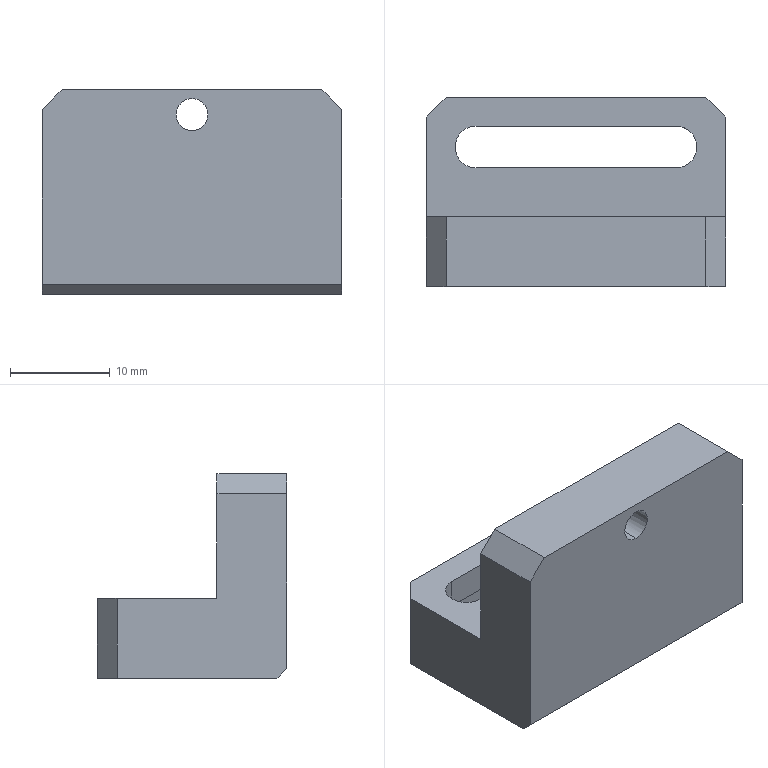Part | SolidWorks | features ICE 4, Chamfer 2, HoleWzd 2, Extrusion 1 | 1 solid | 31 faces | box 30 x 19 x 20.5 mm | volume 5581 mm3 | plane 19 | cylinder 12 | commonest cylinder face diameters 4.2 x3 8 x3 2.5 x2 3.2 x2 3.5 x2
STEP:
#1=CARTESIAN_POINT('',(1.25,-6.,17.001));
#2=VERTEX_POINT('',#1);
#3=CARTESIAN_POINT('',(0.,-7.25,16.4));
#4=VERTEX_POINT('',#3);
#5=CARTESIAN_POINT('',(1.25,-6.,17.001));
#6=CARTESIAN_POINT('',(1.25,-6.086,17.001));
#7=CARTESIAN_POINT('',(1.241,-6.173,16.99));
#8=CARTESIAN_POINT('',(1.206,-6.338,16.949));
#9=CARTESIAN_POINT('',(1.182,-6.415,16.92));
#10=CARTESIAN_POINT('',(1.087,-6.637,16.823));
#11=CARTESIAN_POINT('',(1.001,-6.765,16.745));
#12=CARTESIAN_POINT('',(0.7798,-6.99,16.597));
#13=CARTESIAN_POINT('',(0.6505,-7.08,16.529));
#14=CARTESIAN_POINT('',(0.4204,-7.18,16.454));
#15=CARTESIAN_POINT('',(0.3405,-7.206,16.434));
#16=CARTESIAN_POINT('',(0.1734,-7.241,16.407));
#17=CARTESIAN_POINT('',(0.08602,-7.25,16.4));
#18=CARTESIAN_POINT('',(0.,-7.25,16.4));
#19=B_SPLINE_CURVE_WITH_KNOTS('',3,(#5,#6,#7,#8,#9,#10,#11,#12,#13,#14,#15,#16,#17,#18),.UNSPECIFIED.,.F.,.F.,(4,2,2,2,2,2,4),(0.002061,0.002319,0.002576,0.003092,0.003607,0.003864,0.004122),.UNSPECIFIED.);
#20=EDGE_CURVE('',#2,#4,#19,.T.);
#21=ORIENTED_EDGE('',*,*,#20,.F.);
#22=CARTESIAN_POINT('',(1.25,-6.,10.));
#23=VERTEX_POINT('',#22);
#24=CARTESIAN_POINT('',(1.25,-6.,10.));
#25=DIRECTION('',(0.,0.,-1.));
#26=VECTOR('',#25,1000.);
#27=LINE('',#24,#26);
#28=EDGE_CURVE('',#2,#23,#27,.T.);
#29=ORIENTED_EDGE('',*,*,#28,.T.);
#30=CARTESIAN_POINT('',(-1.25,-6.,10.));
#31=VERTEX_POINT('',#30);
#32=CARTESIAN_POINT('',(0.,-6.,10.));
#33=DIRECTION('',(0.,0.,-1.));
#34=DIRECTION('',(-1.,0.,0.));
#35=AXIS2_PLACEMENT_3D('',#32,#33,#34);
#36=CIRCLE('',#35,1.25);
#37=EDGE_CURVE('',#23,#31,#36,.T.);
#38=ORIENTED_EDGE('',*,*,#37,.T.);
#39=CARTESIAN_POINT('',(-1.25,-6.,17.001));
#40=VERTEX_POINT('',#39);
#41=CARTESIAN_POINT('',(-1.25,-6.,10.));
#42=DIRECTION('',(0.,0.,-1.));
#43=VECTOR('',#42,1000.);
#44=LINE('',#41,#43);
#45=EDGE_CURVE('',#40,#31,#44,.T.);
#46=ORIENTED_EDGE('',*,*,#45,.F.);
#47=CARTESIAN_POINT('',(0.,-7.25,16.4));
#48=CARTESIAN_POINT('',(-0.08574,-7.25,16.4));
#49=CARTESIAN_POINT('',(-0.1725,-7.241,16.407));
#50=CARTESIAN_POINT('',(-0.3395,-7.206,16.434));
#51=CARTESIAN_POINT('',(-0.4194,-7.18,16.454));
#52=CARTESIAN_POINT('',(-0.6488,-7.081,16.529));
#53=CARTESIAN_POINT('',(-0.781,-6.988,16.597));
#54=CARTESIAN_POINT('',(-0.9998,-6.766,16.744));
#55=CARTESIAN_POINT('',(-1.088,-6.636,16.823));
#56=CARTESIAN_POINT('',(-1.213,-6.343,16.952));
#57=CARTESIAN_POINT('',(-1.25,-6.173,17.001));
#58=CARTESIAN_POINT('',(-1.25,-6.,17.001));
#59=B_SPLINE_CURVE_WITH_KNOTS('',3,(#47,#48,#49,#50,#51,#52,#53,#54,#55,#56,#57,#58),.UNSPECIFIED.,.F.,.F.,(4,2,2,2,2,4),(0.004122,0.004379,0.004636,0.005149,0.005663,0.006177),.UNSPECIFIED.);
#60=EDGE_CURVE('',#4,#40,#59,.T.);
#61=ORIENTED_EDGE('',*,*,#60,.F.);
#62=EDGE_LOOP('',(#21,#29,#38,#46,#61));
#63=FACE_OUTER_BOUND('',#62,.T.);
#64=CARTESIAN_POINT('',(0.,-6.,10.));
#65=DIRECTION('',(0.,0.,-1.));
#66=DIRECTION('',(-1.,0.,0.));
#67=AXIS2_PLACEMENT_3D('',#64,#65,#66);
#68=CYLINDRICAL_SURFACE('',#67,1.25);
#69=ADVANCED_FACE('',(#63),#68,.F.);
#70=CARTESIAN_POINT('',(0.,-2.5,19.6));
#71=VERTEX_POINT('',#70);
#72=CARTESIAN_POINT('',(0.,-2.5,16.4));
#73=VERTEX_POINT('',#72);
#74=CARTESIAN_POINT('',(0.,-2.5,18.));
#75=DIRECTION('',(0.,-1.,0.));
#76=DIRECTION('',(0.,0.,-1.));
#77=AXIS2_PLACEMENT_3D('',#74,#75,#76);
#78=CIRCLE('',#77,1.6);
#79=EDGE_CURVE('',#71,#73,#78,.T.);
#80=ORIENTED_EDGE('',*,*,#79,.F.);
#81=CARTESIAN_POINT('',(0.,-9.5,19.6));
#82=VERTEX_POINT('',#81);
#83=CARTESIAN_POINT('',(0.,-9.5,19.6));
#84=DIRECTION('',(0.,-1.,0.));
#85=VECTOR('',#84,1000.);
#86=LINE('',#83,#85);
#87=EDGE_CURVE('',#71,#82,#86,.T.);
#88=ORIENTED_EDGE('',*,*,#87,.T.);
#89=CARTESIAN_POINT('',(0.,-9.5,16.4));
#90=VERTEX_POINT('',#89);
#91=CARTESIAN_POINT('',(0.,-9.5,18.));
#92=DIRECTION('',(0.,-1.,0.));
#93=DIRECTION('',(0.,0.,-1.));
#94=AXIS2_PLACEMENT_3D('',#91,#92,#93);
#95=CIRCLE('',#94,1.6);
#96=EDGE_CURVE('',#82,#90,#95,.T.);
#97=ORIENTED_EDGE('',*,*,#96,.T.);
#98=CARTESIAN_POINT('',(0.,-9.5,16.4));
#99=DIRECTION('',(0.,-1.,0.));
#100=VECTOR('',#99,1000.);
#101=LINE('',#98,#100);
#102=EDGE_CURVE('',#4,#90,#101,.T.);
#103=ORIENTED_EDGE('',*,*,#102,.F.);
#104=ORIENTED_EDGE('',*,*,#60,.T.);
#105=CARTESIAN_POINT('',(0.,-4.75,16.4));
#106=VERTEX_POINT('',#105);
#107=CARTESIAN_POINT('',(-1.25,-6.,17.001));
#108=CARTESIAN_POINT('',(-1.25,-5.913,17.001));
#109=CARTESIAN_POINT('',(-1.241,-5.828,16.99));
#110=CARTESIAN_POINT('',(-1.206,-5.662,16.949));
#111=CARTESIAN_POINT('',(-1.182,-5.585,16.92));
#112=CARTESIAN_POINT('',(-1.088,-5.363,16.823));
#113=CARTESIAN_POINT('',(-1.001,-5.235,16.745));
#114=CARTESIAN_POINT('',(-0.7808,-5.011,16.597));
#115=CARTESIAN_POINT('',(-0.6506,-4.92,16.529));
#116=CARTESIAN_POINT('',(-0.3461,-4.787,16.43));
#117=CARTESIAN_POINT('',(-0.1743,-4.75,16.4));
#118=CARTESIAN_POINT('',(0.,-4.75,16.4));
#119=B_SPLINE_CURVE_WITH_KNOTS('',3,(#107,#108,#109,#110,#111,#112,#113,#114,#115,#116,#117,#118),.UNSPECIFIED.,.F.,.F.,(4,2,2,2,2,4),(0.006177,0.006434,0.006691,0.007205,0.00772,0.008234),.UNSPECIFIED.);
#120=EDGE_CURVE('',#40,#106,#119,.T.);
#121=ORIENTED_EDGE('',*,*,#120,.T.);
#122=CARTESIAN_POINT('',(0.,-9.5,16.4));
#123=DIRECTION('',(0.,-1.,0.));
#124=VECTOR('',#123,1000.);
#125=LINE('',#122,#124);
#126=EDGE_CURVE('',#73,#106,#125,.T.);
#127=ORIENTED_EDGE('',*,*,#126,.F.);
#128=EDGE_LOOP('',(#80,#88,#97,#103,#104,#121,#127));
#129=FACE_OUTER_BOUND('',#128,.T.);
#130=CARTESIAN_POINT('',(0.,-9.5,18.));
#131=DIRECTION('',(0.,-1.,0.));
#132=DIRECTION('',(0.,0.,-1.));
#133=AXIS2_PLACEMENT_3D('',#130,#131,#132);
#134=CYLINDRICAL_SURFACE('',#133,1.6);
#135=ADVANCED_FACE('',(#129),#134,.F.);
#136=CARTESIAN_POINT('',(1.75,-6.,10.));
#137=VERTEX_POINT('',#136);
#138=CARTESIAN_POINT('',(-1.75,-6.,10.));
#139=VERTEX_POINT('',#138);
#140=CARTESIAN_POINT('',(0.,-6.,10.));
#141=DIRECTION('',(0.,0.,-1.));
#142=DIRECTION('',(-1.,0.,0.));
#143=AXIS2_PLACEMENT_3D('',#140,#141,#142);
#144=CIRCLE('',#143,1.75);
#145=EDGE_CURVE('',#137,#139,#144,.T.);
#146=ORIENTED_EDGE('',*,*,#145,.F.);
#147=CARTESIAN_POINT('',(1.75,-6.,0.));
#148=VERTEX_POINT('',#147);
#149=CARTESIAN_POINT('',(1.75,-6.,10.));
#150=DIRECTION('',(0.,0.,-1.));
#151=VECTOR('',#150,1000.);
#152=LINE('',#149,#151);
#153=EDGE_CURVE('',#137,#148,#152,.T.);
#154=ORIENTED_EDGE('',*,*,#153,.T.);
#155=CARTESIAN_POINT('',(-1.75,-6.,0.));
#156=VERTEX_POINT('',#155);
#157=CARTESIAN_POINT('',(0.,-6.,0.));
#158=DIRECTION('',(0.,0.,-1.));
#159=DIRECTION('',(-1.,0.,0.));
#160=AXIS2_PLACEMENT_3D('',#157,#158,#159);
#161=CIRCLE('',#160,1.75);
#162=EDGE_CURVE('',#148,#156,#161,.T.);
#163=ORIENTED_EDGE('',*,*,#162,.T.);
#164=CARTESIAN_POINT('',(-1.75,-6.,10.));
#165=DIRECTION('',(0.,0.,-1.));
#166=VECTOR('',#165,1000.);
#167=LINE('',#164,#166);
#168=EDGE_CURVE('',#139,#156,#167,.T.);
#169=ORIENTED_EDGE('',*,*,#168,.F.);
#170=EDGE_LOOP('',(#146,#154,#163,#169));
#171=FACE_OUTER_BOUND('',#170,.T.);
#172=CARTESIAN_POINT('',(0.,-6.,10.));
#173=DIRECTION('',(0.,0.,-1.));
#174=DIRECTION('',(-1.,0.,0.));
#175=AXIS2_PLACEMENT_3D('',#172,#173,#174);
#176=CYLINDRICAL_SURFACE('',#175,1.75);
#177=ADVANCED_FACE('',(#171),#176,.F.);
#178=CARTESIAN_POINT('',(-14.,4.5,5.));
#179=VERTEX_POINT('',#178);
#180=CARTESIAN_POINT('',(-10.,8.5,5.));
#181=VERTEX_POINT('',#180);
#182=CARTESIAN_POINT('',(-10.,4.5,5.));
#183=DIRECTION('',(0.,0.,-1.));
#184=DIRECTION('',(-1.,0.,0.));
#185=AXIS2_PLACEMENT_3D('',#182,#183,#184);
#186=CIRCLE('',#185,4.);
#187=EDGE_CURVE('',#179,#181,#186,.T.);
#188=ORIENTED_EDGE('',*,*,#187,.F.);
#189=CARTESIAN_POINT('',(-14.,4.5,0.));
#190=VERTEX_POINT('',#189);
#191=CARTESIAN_POINT('',(-14.,4.5,5.));
#192=DIRECTION('',(0.,0.,-1.));
#193=VECTOR('',#192,1000.);
#194=LINE('',#191,#193);
#195=EDGE_CURVE('',#179,#190,#194,.T.);
#196=ORIENTED_EDGE('',*,*,#195,.T.);
#197=CARTESIAN_POINT('',(-10.,8.5,0.));
#198=VERTEX_POINT('',#197);
#199=CARTESIAN_POINT('',(-10.,4.5,0.));
#200=DIRECTION('',(0.,0.,-1.));
#201=DIRECTION('',(-1.,0.,0.));
#202=AXIS2_PLACEMENT_3D('',#199,#200,#201);
#203=CIRCLE('',#202,4.);
#204=EDGE_CURVE('',#190,#198,#203,.T.);
#205=ORIENTED_EDGE('',*,*,#204,.T.);
#206=CARTESIAN_POINT('',(-10.,8.5,5.));
#207=DIRECTION('',(0.,0.,-1.));
#208=VECTOR('',#207,1000.);
#209=LINE('',#206,#208);
#210=EDGE_CURVE('',#181,#198,#209,.T.);
#211=ORIENTED_EDGE('',*,*,#210,.F.);
#212=EDGE_LOOP('',(#188,#196,#205,#211));
#213=FACE_OUTER_BOUND('',#212,.T.);
#214=CARTESIAN_POINT('',(-10.,4.5,5.));
#215=DIRECTION('',(0.,0.,-1.));
#216=DIRECTION('',(-1.,0.,0.));
#217=AXIS2_PLACEMENT_3D('',#214,#215,#216);
#218=CYLINDRICAL_SURFACE('',#217,4.);
#219=ADVANCED_FACE('',(#213),#218,.F.);
#220=CARTESIAN_POINT('',(-10.,6.6,8.));
#221=VERTEX_POINT('',#220);
#222=CARTESIAN_POINT('',(-12.1,4.5,8.));
#223=VERTEX_POINT('',#222);
#224=CARTESIAN_POINT('',(-10.,4.5,8.));
#225=DIRECTION('',(0.,0.,1.));
#226=DIRECTION('',(1.,0.,0.));
#227=AXIS2_PLACEMENT_3D('',#224,#225,#226);
#228=CIRCLE('',#227,2.1);
#229=EDGE_CURVE('',#221,#223,#228,.T.);
#230=ORIENTED_EDGE('',*,*,#229,.T.);
#231=CARTESIAN_POINT('',(-12.1,4.5,5.));
#232=VERTEX_POINT('',#231);
#233=CARTESIAN_POINT('',(-12.1,4.5,20.5));
#234=DIRECTION('',(0.,0.,-1.));
#235=VECTOR('',#234,1000.);
#236=LINE('',#233,#235);
#237=EDGE_CURVE('',#223,#232,#236,.T.);
#238=ORIENTED_EDGE('',*,*,#237,.T.);
#239=CARTESIAN_POINT('',(-10.,6.6,5.));
#240=VERTEX_POINT('',#239);
#241=CARTESIAN_POINT('',(-10.,4.5,5.));
#242=DIRECTION('',(0.,0.,1.));
#243=DIRECTION('',(-1.,0.,0.));
#244=AXIS2_PLACEMENT_3D('',#241,#242,#243);
#245=CIRCLE('',#244,2.1);
#246=EDGE_CURVE('',#240,#232,#245,.T.);
#247=ORIENTED_EDGE('',*,*,#246,.F.);
#248=CARTESIAN_POINT('',(-10.,6.6,20.5));
#249=DIRECTION('',(0.,0.,-1.));
#250=VECTOR('',#249,1000.);
#251=LINE('',#248,#250);
#252=EDGE_CURVE('',#221,#240,#251,.T.);
#253=ORIENTED_EDGE('',*,*,#252,.F.);
#254=EDGE_LOOP('',(#230,#238,#247,#253));
#255=FACE_OUTER_BOUND('',#254,.T.);
#256=CARTESIAN_POINT('',(-10.,4.5,20.5));
#257=DIRECTION('',(0.,0.,-1.));
#258=DIRECTION('',(-1.,0.,0.));
#259=AXIS2_PLACEMENT_3D('',#256,#257,#258);
#260=CYLINDRICAL_SURFACE('',#259,2.1);
#261=ADVANCED_FACE('',(#255),#260,.F.);
#262=ORIENTED_EDGE('',*,*,#237,.F.);
#263=CARTESIAN_POINT('',(-10.,2.4,8.));
#264=VERTEX_POINT('',#263);
#265=CARTESIAN_POINT('',(-10.,4.5,8.));
#266=DIRECTION('',(0.,0.,1.));
#267=DIRECTION('',(1.,0.,0.));
#268=AXIS2_PLACEMENT_3D('',#265,#266,#267);
#269=CIRCLE('',#268,2.1);
#270=EDGE_CURVE('',#223,#264,#269,.T.);
#271=ORIENTED_EDGE('',*,*,#270,.T.);
#272=CARTESIAN_POINT('',(-10.,2.4,5.));
#273=VERTEX_POINT('',#272);
#274=CARTESIAN_POINT('',(-10.,2.4,20.5));
#275=DIRECTION('',(0.,0.,-1.));
#276=VECTOR('',#275,1000.);
#277=LINE('',#274,#276);
#278=EDGE_CURVE('',#264,#273,#277,.T.);
#279=ORIENTED_EDGE('',*,*,#278,.T.);
#280=CARTESIAN_POINT('',(-10.,4.5,5.));
#281=DIRECTION('',(0.,0.,1.));
#282=DIRECTION('',(-1.,0.,0.));
#283=AXIS2_PLACEMENT_3D('',#280,#281,#282);
#284=CIRCLE('',#283,2.1);
#285=EDGE_CURVE('',#232,#273,#284,.T.);
#286=ORIENTED_EDGE('',*,*,#285,.F.);
#287=EDGE_LOOP('',(#262,#271,#279,#286));
#288=FACE_OUTER_BOUND('',#287,.T.);
#289=CARTESIAN_POINT('',(-10.,4.5,20.5));
#290=DIRECTION('',(0.,0.,-1.));
#291=DIRECTION('',(-1.,0.,0.));
#292=AXIS2_PLACEMENT_3D('',#289,#290,#291);
#293=CYLINDRICAL_SURFACE('',#292,2.1);
#294=ADVANCED_FACE('',(#288),#293,.F.);
#295=CARTESIAN_POINT('',(10.,2.4,5.));
#296=VERTEX_POINT('',#295);
#297=CARTESIAN_POINT('',(-10.,2.4,5.));
#298=DIRECTION('',(1.,0.,0.));
#299=VECTOR('',#298,1000.);
#300=LINE('',#297,#299);
#301=EDGE_CURVE('',#273,#296,#300,.T.);
#302=ORIENTED_EDGE('',*,*,#301,.F.);
#303=ORIENTED_EDGE('',*,*,#278,.F.);
#304=CARTESIAN_POINT('',(10.,2.4,8.));
#305=VERTEX_POINT('',#304);
#306=CARTESIAN_POINT('',(0.,2.4,8.));
#307=DIRECTION('',(1.,0.,0.));
#308=VECTOR('',#307,1000.);
#309=LINE('',#306,#308);
#310=EDGE_CURVE('',#264,#305,#309,.T.);
#311=ORIENTED_EDGE('',*,*,#310,.T.);
#312=CARTESIAN_POINT('',(10.,2.4,20.5));
#313=DIRECTION('',(0.,0.,-1.));
#314=VECTOR('',#313,1000.);
#315=LINE('',#312,#314);
#316=EDGE_CURVE('',#305,#296,#315,.T.);
#317=ORIENTED_EDGE('',*,*,#316,.T.);
#318=EDGE_LOOP('',(#302,#303,#311,#317));
#319=FACE_OUTER_BOUND('',#318,.T.);
#320=CARTESIAN_POINT('',(-10.,2.4,20.5));
#321=DIRECTION('',(0.,-1.,0.));
#322=DIRECTION('',(1.,0.,0.));
#323=AXIS2_PLACEMENT_3D('',#320,#321,#322);
#324=PLANE('',#323);
#325=ADVANCED_FACE('',(#319),#324,.F.);
#326=CARTESIAN_POINT('',(10.,6.6,5.));
#327=VERTEX_POINT('',#326);
#328=CARTESIAN_POINT('',(10.,4.5,5.));
#329=DIRECTION('',(0.,0.,1.));
#330=DIRECTION('',(-1.,0.,0.));
#331=AXIS2_PLACEMENT_3D('',#328,#329,#330);
#332=CIRCLE('',#331,2.1);
#333=EDGE_CURVE('',#296,#327,#332,.T.);
#334=ORIENTED_EDGE('',*,*,#333,.F.);
#335=ORIENTED_EDGE('',*,*,#316,.F.);
#336=CARTESIAN_POINT('',(10.,6.6,8.));
#337=VERTEX_POINT('',#336);
#338=CARTESIAN_POINT('',(10.,4.5,8.));
#339=DIRECTION('',(0.,0.,1.));
#340=DIRECTION('',(1.,0.,0.));
#341=AXIS2_PLACEMENT_3D('',#338,#339,#340);
#342=CIRCLE('',#341,2.1);
#343=EDGE_CURVE('',#305,#337,#342,.T.);
#344=ORIENTED_EDGE('',*,*,#343,.T.);
#345=CARTESIAN_POINT('',(10.,6.6,20.5));
#346=DIRECTION('',(0.,0.,-1.));
#347=VECTOR('',#346,1000.);
#348=LINE('',#345,#347);
#349=EDGE_CURVE('',#337,#327,#348,.T.);
#350=ORIENTED_EDGE('',*,*,#349,.T.);
#351=EDGE_LOOP('',(#334,#335,#344,#350));
#352=FACE_OUTER_BOUND('',#351,.T.);
#353=CARTESIAN_POINT('',(10.,4.5,20.5));
#354=DIRECTION('',(0.,0.,-1.));
#355=DIRECTION('',(-1.,0.,0.));
#356=AXIS2_PLACEMENT_3D('',#353,#354,#355);
#357=CYLINDRICAL_SURFACE('',#356,2.1);
#358=ADVANCED_FACE('',(#352),#357,.F.);
#359=CARTESIAN_POINT('',(-10.,6.6,5.));
#360=DIRECTION('',(-1.,0.,0.));
#361=VECTOR('',#360,1000.);
#362=LINE('',#359,#361);
#363=EDGE_CURVE('',#327,#240,#362,.T.);
#364=ORIENTED_EDGE('',*,*,#363,.F.);
#365=ORIENTED_EDGE('',*,*,#349,.F.);
#366=CARTESIAN_POINT('',(0.,6.6,8.));
#367=DIRECTION('',(-1.,0.,0.));
#368=VECTOR('',#367,1000.);
#369=LINE('',#366,#368);
#370=EDGE_CURVE('',#337,#221,#369,.T.);
#371=ORIENTED_EDGE('',*,*,#370,.T.);
#372=ORIENTED_EDGE('',*,*,#252,.T.);
#373=EDGE_LOOP('',(#364,#365,#371,#372));
#374=FACE_OUTER_BOUND('',#373,.T.);
#375=CARTESIAN_POINT('',(-10.,6.6,20.5));
#376=DIRECTION('',(0.,1.,0.));
#377=DIRECTION('',(-1.,0.,0.));
#378=AXIS2_PLACEMENT_3D('',#375,#376,#377);
#379=PLANE('',#378);
#380=ADVANCED_FACE('',(#374),#379,.F.);
#381=CARTESIAN_POINT('',(13.,9.5,0.));
#382=VERTEX_POINT('',#381);
#383=CARTESIAN_POINT('',(-13.,9.5,0.));
#384=VERTEX_POINT('',#383);
#385=CARTESIAN_POINT('',(-15.,9.5,0.));
#386=DIRECTION('',(-1.,0.,0.));
#387=VECTOR('',#386,1000.);
#388=LINE('',#385,#387);
#389=EDGE_CURVE('',#382,#384,#388,.T.);
#390=ORIENTED_EDGE('',*,*,#389,.T.);
#391=CARTESIAN_POINT('',(-13.,9.5,8.));
#392=VERTEX_POINT('',#391);
#393=CARTESIAN_POINT('',(-13.,9.5,20.5));
#394=DIRECTION('',(0.,0.,1.));
#395=VECTOR('',#394,1000.);
#396=LINE('',#393,#395);
#397=EDGE_CURVE('',#384,#392,#396,.T.);
#398=ORIENTED_EDGE('',*,*,#397,.T.);
#399=CARTESIAN_POINT('',(13.,9.5,8.));
#400=VERTEX_POINT('',#399);
#401=CARTESIAN_POINT('',(-15.,9.5,8.));
#402=DIRECTION('',(-1.,0.,0.));
#403=VECTOR('',#402,1000.);
#404=LINE('',#401,#403);
#405=EDGE_CURVE('',#400,#392,#404,.T.);
#406=ORIENTED_EDGE('',*,*,#405,.F.);
#407=CARTESIAN_POINT('',(13.,9.5,20.5));
#408=DIRECTION('',(0.,0.,-1.));
#409=VECTOR('',#408,1000.);
#410=LINE('',#407,#409);
#411=EDGE_CURVE('',#400,#382,#410,.T.);
#412=ORIENTED_EDGE('',*,*,#411,.T.);
#413=EDGE_LOOP('',(#390,#398,#406,#412));
#414=FACE_OUTER_BOUND('',#413,.T.);
#415=CARTESIAN_POINT('',(-15.,9.5,20.5));
#416=DIRECTION('',(0.,-1.,0.));
#417=DIRECTION('',(0.,0.,-1.));
#418=AXIS2_PLACEMENT_3D('',#415,#416,#417);
#419=PLANE('',#418);
#420=ADVANCED_FACE('',(#414),#419,.F.);
#421=CARTESIAN_POINT('',(15.,-9.5,18.5));
#422=VERTEX_POINT('',#421);
#423=CARTESIAN_POINT('',(15.,-9.5,1.));
#424=VERTEX_POINT('',#423);
#425=CARTESIAN_POINT('',(15.,-9.5,20.5));
#426=DIRECTION('',(0.,0.,-1.));
#427=VECTOR('',#426,1000.);
#428=LINE('',#425,#427);
#429=EDGE_CURVE('',#422,#424,#428,.T.);
#430=ORIENTED_EDGE('',*,*,#429,.T.);
#431=CARTESIAN_POINT('',(15.,-8.5,0.));
#432=VERTEX_POINT('',#431);
#433=CARTESIAN_POINT('',(15.,-9.5,1.));
#434=DIRECTION('',(0.,0.7071,-0.7071));
#435=VECTOR('',#434,1000.);
#436=LINE('',#433,#435);
#437=EDGE_CURVE('',#424,#432,#436,.T.);
#438=ORIENTED_EDGE('',*,*,#437,.T.);
#439=CARTESIAN_POINT('',(15.,7.5,0.));
#440=VERTEX_POINT('',#439);
#441=CARTESIAN_POINT('',(15.,-9.5,0.));
#442=DIRECTION('',(0.,1.,0.));
#443=VECTOR('',#442,1000.);
#444=LINE('',#441,#443);
#445=EDGE_CURVE('',#432,#440,#444,.T.);
#446=ORIENTED_EDGE('',*,*,#445,.T.);
#447=CARTESIAN_POINT('',(15.,7.5,8.));
#448=VERTEX_POINT('',#447);
#449=CARTESIAN_POINT('',(15.,7.5,20.5));
#450=DIRECTION('',(0.,0.,1.));
#451=VECTOR('',#450,1000.);
#452=LINE('',#449,#451);
#453=EDGE_CURVE('',#440,#448,#452,.T.);
#454=ORIENTED_EDGE('',*,*,#453,.T.);
#455=CARTESIAN_POINT('',(15.,-2.5,8.));
#456=VERTEX_POINT('',#455);
#457=CARTESIAN_POINT('',(15.,9.5,8.));
#458=DIRECTION('',(0.,1.,0.));
#459=VECTOR('',#458,1000.);
#460=LINE('',#457,#459);
#461=EDGE_CURVE('',#456,#448,#460,.T.);
#462=ORIENTED_EDGE('',*,*,#461,.F.);
#463=CARTESIAN_POINT('',(15.,-2.5,18.5));
#464=VERTEX_POINT('',#463);
#465=CARTESIAN_POINT('',(15.,-2.5,8.));
#466=DIRECTION('',(0.,0.,1.));
#467=VECTOR('',#466,1000.);
#468=LINE('',#465,#467);
#469=EDGE_CURVE('',#456,#464,#468,.T.);
#470=ORIENTED_EDGE('',*,*,#469,.T.);
#471=CARTESIAN_POINT('',(15.,-9.5,18.5));
#472=DIRECTION('',(0.,-1.,0.));
#473=VECTOR('',#472,1000.);
#474=LINE('',#471,#473);
#475=EDGE_CURVE('',#464,#422,#474,.T.);
#476=ORIENTED_EDGE('',*,*,#475,.T.);
#477=EDGE_LOOP('',(#430,#438,#446,#454,#462,#470,#476));
#478=FACE_OUTER_BOUND('',#477,.T.);
#479=CARTESIAN_POINT('',(15.,-9.5,20.5));
#480=DIRECTION('',(-1.,0.,0.));
#481=DIRECTION('',(0.,0.,1.));
#482=AXIS2_PLACEMENT_3D('',#479,#480,#481);
#483=PLANE('',#482);
#484=ADVANCED_FACE('',(#478),#483,.F.);
#485=CARTESIAN_POINT('',(-15.,7.5,0.));
#486=VERTEX_POINT('',#485);
#487=CARTESIAN_POINT('',(-15.,-8.5,0.));
#488=VERTEX_POINT('',#487);
#489=CARTESIAN_POINT('',(-15.,-9.5,0.));
#490=DIRECTION('',(0.,-1.,0.));
#491=VECTOR('',#490,1000.);
#492=LINE('',#489,#491);
#493=EDGE_CURVE('',#486,#488,#492,.T.);
#494=ORIENTED_EDGE('',*,*,#493,.T.);
#495=CARTESIAN_POINT('',(-15.,-9.5,1.));
#496=VERTEX_POINT('',#495);
#497=CARTESIAN_POINT('',(-15.,-9.5,1.));
#498=DIRECTION('',(0.,-0.7071,0.7071));
#499=VECTOR('',#498,1000.);
#500=LINE('',#497,#499);
#501=EDGE_CURVE('',#488,#496,#500,.T.);
#502=ORIENTED_EDGE('',*,*,#501,.T.);
#503=CARTESIAN_POINT('',(-15.,-9.5,18.5));
#504=VERTEX_POINT('',#503);
#505=CARTESIAN_POINT('',(-15.,-9.5,20.5));
#506=DIRECTION('',(0.,0.,-1.));
#507=VECTOR('',#506,1000.);
#508=LINE('',#505,#507);
#509=EDGE_CURVE('',#504,#496,#508,.T.);
#510=ORIENTED_EDGE('',*,*,#509,.F.);
#511=CARTESIAN_POINT('',(-15.,-2.5,18.5));
#512=VERTEX_POINT('',#511);
#513=CARTESIAN_POINT('',(-15.,-9.5,18.5));
#514=DIRECTION('',(0.,1.,0.));
#515=VECTOR('',#514,1000.);
#516=LINE('',#513,#515);
#517=EDGE_CURVE('',#504,#512,#516,.T.);
#518=ORIENTED_EDGE('',*,*,#517,.T.);
#519=CARTESIAN_POINT('',(-15.,-2.5,8.));
#520=VERTEX_POINT('',#519);
#521=CARTESIAN_POINT('',(-15.,-2.5,8.));
#522=DIRECTION('',(0.,0.,1.));
#523=VECTOR('',#522,1000.);
#524=LINE('',#521,#523);
#525=EDGE_CURVE('',#520,#512,#524,.T.);
#526=ORIENTED_EDGE('',*,*,#525,.F.);
#527=CARTESIAN_POINT('',(-15.,7.5,8.));
#528=VERTEX_POINT('',#527);
#529=CARTESIAN_POINT('',(-15.,9.5,8.));
#530=DIRECTION('',(0.,-1.,0.));
#531=VECTOR('',#530,1000.);
#532=LINE('',#529,#531);
#533=EDGE_CURVE('',#528,#520,#532,.T.);
#534=ORIENTED_EDGE('',*,*,#533,.F.);
#535=CARTESIAN_POINT('',(-15.,7.5,20.5));
#536=DIRECTION('',(0.,0.,-1.));
#537=VECTOR('',#536,1000.);
#538=LINE('',#535,#537);
#539=EDGE_CURVE('',#528,#486,#538,.T.);
#540=ORIENTED_EDGE('',*,*,#539,.T.);
#541=EDGE_LOOP('',(#494,#502,#510,#518,#526,#534,#540));
#542=FACE_OUTER_BOUND('',#541,.T.);
#543=CARTESIAN_POINT('',(-15.,-9.5,20.5));
#544=DIRECTION('',(1.,0.,0.));
#545=DIRECTION('',(0.,0.,-1.));
#546=AXIS2_PLACEMENT_3D('',#543,#544,#545);
#547=PLANE('',#546);
#548=ADVANCED_FACE('',(#542),#547,.F.);
#549=CARTESIAN_POINT('',(0.,-9.5,18.));
#550=DIRECTION('',(0.,-1.,0.));
#551=DIRECTION('',(0.,0.,-1.));
#552=AXIS2_PLACEMENT_3D('',#549,#550,#551);
#553=CIRCLE('',#552,1.6);
#554=EDGE_CURVE('',#90,#82,#553,.T.);
#555=ORIENTED_EDGE('',*,*,#554,.F.);
#556=ORIENTED_EDGE('',*,*,#96,.F.);
#557=EDGE_LOOP('',(#555,#556));
#558=FACE_BOUND('',#557,.T.);
#559=ORIENTED_EDGE('',*,*,#509,.T.);
#560=CARTESIAN_POINT('',(15.,-9.5,1.));
#561=DIRECTION('',(1.,0.,0.));
#562=VECTOR('',#561,1000.);
#563=LINE('',#560,#562);
#564=EDGE_CURVE('',#496,#424,#563,.T.);
#565=ORIENTED_EDGE('',*,*,#564,.T.);
#566=ORIENTED_EDGE('',*,*,#429,.F.);
#567=CARTESIAN_POINT('',(13.,-9.5,20.5));
#568=VERTEX_POINT('',#567);
#569=CARTESIAN_POINT('',(13.,-9.5,20.5));
#570=DIRECTION('',(-0.7071,0.,0.7071));
#571=VECTOR('',#570,1000.);
#572=LINE('',#569,#571);
#573=EDGE_CURVE('',#422,#568,#572,.T.);
#574=ORIENTED_EDGE('',*,*,#573,.T.);
#575=CARTESIAN_POINT('',(-13.,-9.5,20.5));
#576=VERTEX_POINT('',#575);
#577=CARTESIAN_POINT('',(-15.,-9.5,20.5));
#578=DIRECTION('',(1.,0.,0.));
#579=VECTOR('',#578,1000.);
#580=LINE('',#577,#579);
#581=EDGE_CURVE('',#576,#568,#580,.T.);
#582=ORIENTED_EDGE('',*,*,#581,.F.);
#583=CARTESIAN_POINT('',(-13.,-9.5,20.5));
#584=DIRECTION('',(-0.7071,0.,-0.7071));
#585=VECTOR('',#584,1000.);
#586=LINE('',#583,#585);
#587=EDGE_CURVE('',#576,#504,#586,.T.);
#588=ORIENTED_EDGE('',*,*,#587,.T.);
#589=EDGE_LOOP('',(#559,#565,#566,#574,#582,#588));
#590=FACE_OUTER_BOUND('',#589,.T.);
#591=CARTESIAN_POINT('',(-15.,-9.5,20.5));
#592=DIRECTION('',(0.,1.,0.));
#593=DIRECTION('',(0.,0.,1.));
#594=AXIS2_PLACEMENT_3D('',#591,#592,#593);
#595=PLANE('',#594);
#596=ADVANCED_FACE('',(#558,#590),#595,.F.);
#597=ORIENTED_EDGE('',*,*,#581,.T.);
#598=CARTESIAN_POINT('',(13.,-2.5,20.5));
#599=VERTEX_POINT('',#598);
#600=CARTESIAN_POINT('',(13.,0.,20.5));
#601=DIRECTION('',(0.,1.,0.));
#602=VECTOR('',#601,1000.);
#603=LINE('',#600,#602);
#604=EDGE_CURVE('',#568,#599,#603,.T.);
#605=ORIENTED_EDGE('',*,*,#604,.T.);
#606=CARTESIAN_POINT('',(-13.,-2.5,20.5));
#607=VERTEX_POINT('',#606);
#608=CARTESIAN_POINT('',(-15.,-2.5,20.5));
#609=DIRECTION('',(1.,0.,0.));
#610=VECTOR('',#609,1000.);
#611=LINE('',#608,#610);
#612=EDGE_CURVE('',#607,#599,#611,.T.);
#613=ORIENTED_EDGE('',*,*,#612,.F.);
#614=CARTESIAN_POINT('',(-13.,0.,20.5));
#615=DIRECTION('',(0.,-1.,0.));
#616=VECTOR('',#615,1000.);
#617=LINE('',#614,#616);
#618=EDGE_CURVE('',#607,#576,#617,.T.);
#619=ORIENTED_EDGE('',*,*,#618,.T.);
#620=EDGE_LOOP('',(#597,#605,#613,#619));
#621=FACE_OUTER_BOUND('',#620,.T.);
#622=CARTESIAN_POINT('',(0.,0.,20.5));
#623=DIRECTION('',(0.,0.,-1.));
#624=DIRECTION('',(-1.,0.,0.));
#625=AXIS2_PLACEMENT_3D('',#622,#623,#624);
#626=PLANE('',#625);
#627=ADVANCED_FACE('',(#621),#626,.F.);
#628=CARTESIAN_POINT('',(0.,-6.,0.));
#629=DIRECTION('',(0.,0.,-1.));
#630=DIRECTION('',(-1.,0.,0.));
#631=AXIS2_PLACEMENT_3D('',#628,#629,#630);
#632=CIRCLE('',#631,1.75);
#633=EDGE_CURVE('',#156,#148,#632,.T.);
#634=ORIENTED_EDGE('',*,*,#633,.F.);
#635=ORIENTED_EDGE('',*,*,#162,.F.);
#636=EDGE_LOOP('',(#634,#635));
#637=FACE_BOUND('',#636,.T.);
#638=CARTESIAN_POINT('',(-10.,0.5,0.));
#639=VERTEX_POINT('',#638);
#640=CARTESIAN_POINT('',(-10.,4.5,0.));
#641=DIRECTION('',(0.,0.,-1.));
#642=DIRECTION('',(-1.,0.,0.));
#643=AXIS2_PLACEMENT_3D('',#640,#641,#642);
#644=CIRCLE('',#643,4.);
#645=EDGE_CURVE('',#639,#190,#644,.T.);
#646=ORIENTED_EDGE('',*,*,#645,.F.);
#647=CARTESIAN_POINT('',(10.,0.5,0.));
#648=VERTEX_POINT('',#647);
#649=CARTESIAN_POINT('',(-10.,0.5,0.));
#650=DIRECTION('',(-1.,0.,0.));
#651=VECTOR('',#650,1000.);
#652=LINE('',#649,#651);
#653=EDGE_CURVE('',#648,#639,#652,.T.);
#654=ORIENTED_EDGE('',*,*,#653,.F.);
#655=CARTESIAN_POINT('',(10.,8.5,0.));
#656=VERTEX_POINT('',#655);
#657=CARTESIAN_POINT('',(10.,4.5,0.));
#658=DIRECTION('',(0.,0.,-1.));
#659=DIRECTION('',(-1.,0.,0.));
#660=AXIS2_PLACEMENT_3D('',#657,#658,#659);
#661=CIRCLE('',#660,4.);
#662=EDGE_CURVE('',#656,#648,#661,.T.);
#663=ORIENTED_EDGE('',*,*,#662,.F.);
#664=CARTESIAN_POINT('',(-10.,8.5,0.));
#665=DIRECTION('',(1.,0.,0.));
#666=VECTOR('',#665,1000.);
#667=LINE('',#664,#666);
#668=EDGE_CURVE('',#198,#656,#667,.T.);
#669=ORIENTED_EDGE('',*,*,#668,.F.);
#670=ORIENTED_EDGE('',*,*,#204,.F.);
#671=EDGE_LOOP('',(#646,#654,#663,#669,#670));
#672=FACE_BOUND('',#671,.T.);
#673=ORIENTED_EDGE('',*,*,#445,.F.);
#674=CARTESIAN_POINT('',(-15.,-8.5,0.));
#675=DIRECTION('',(-1.,0.,0.));
#676=VECTOR('',#675,1000.);
#677=LINE('',#674,#676);
#678=EDGE_CURVE('',#432,#488,#677,.T.);
#679=ORIENTED_EDGE('',*,*,#678,.T.);
#680=ORIENTED_EDGE('',*,*,#493,.F.);
#681=CARTESIAN_POINT('',(-11.25,11.25,0.));
#682=DIRECTION('',(0.7071,0.7071,0.));
#683=VECTOR('',#682,1000.);
#684=LINE('',#681,#683);
#685=EDGE_CURVE('',#486,#384,#684,.T.);
#686=ORIENTED_EDGE('',*,*,#685,.T.);
#687=ORIENTED_EDGE('',*,*,#389,.F.);
#688=CARTESIAN_POINT('',(11.25,11.25,0.));
#689=DIRECTION('',(0.7071,-0.7071,0.));
#690=VECTOR('',#689,1000.);
#691=LINE('',#688,#690);
#692=EDGE_CURVE('',#382,#440,#691,.T.);
#693=ORIENTED_EDGE('',*,*,#692,.T.);
#694=EDGE_LOOP('',(#673,#679,#680,#686,#687,#693));
#695=FACE_OUTER_BOUND('',#694,.T.);
#696=CARTESIAN_POINT('',(0.,0.,0.));
#697=DIRECTION('',(0.,0.,-1.));
#698=DIRECTION('',(-1.,0.,0.));
#699=AXIS2_PLACEMENT_3D('',#696,#697,#698);
#700=PLANE('',#699);
#701=ADVANCED_FACE('',(#637,#672,#695),#700,.T.);
#702=CARTESIAN_POINT('',(0.,-2.5,18.));
#703=DIRECTION('',(0.,-1.,0.));
#704=DIRECTION('',(0.,0.,-1.));
#705=AXIS2_PLACEMENT_3D('',#702,#703,#704);
#706=CIRCLE('',#705,1.6);
#707=EDGE_CURVE('',#73,#71,#706,.T.);
#708=ORIENTED_EDGE('',*,*,#707,.T.);
#709=ORIENTED_EDGE('',*,*,#79,.T.);
#710=EDGE_LOOP('',(#708,#709));
#711=FACE_BOUND('',#710,.T.);
#712=ORIENTED_EDGE('',*,*,#612,.T.);
#713=CARTESIAN_POINT('',(13.,-2.5,20.5));
#714=DIRECTION('',(0.7071,0.,-0.7071));
#715=VECTOR('',#714,1000.);
#716=LINE('',#713,#715);
#717=EDGE_CURVE('',#599,#464,#716,.T.);
#718=ORIENTED_EDGE('',*,*,#717,.T.);
#719=ORIENTED_EDGE('',*,*,#469,.F.);
#720=CARTESIAN_POINT('',(-15.,-2.5,8.));
#721=DIRECTION('',(1.,0.,0.));
#722=VECTOR('',#721,1000.);
#723=LINE('',#720,#722);
#724=EDGE_CURVE('',#520,#456,#723,.T.);
#725=ORIENTED_EDGE('',*,*,#724,.F.);
#726=ORIENTED_EDGE('',*,*,#525,.T.);
#727=CARTESIAN_POINT('',(-13.,-2.5,20.5));
#728=DIRECTION('',(0.7071,0.,0.7071));
#729=VECTOR('',#728,1000.);
#730=LINE('',#727,#729);
#731=EDGE_CURVE('',#512,#607,#730,.T.);
#732=ORIENTED_EDGE('',*,*,#731,.T.);
#733=EDGE_LOOP('',(#712,#718,#719,#725,#726,#732));
#734=FACE_OUTER_BOUND('',#733,.T.);
#735=CARTESIAN_POINT('',(-15.,-2.5,8.));
#736=DIRECTION('',(0.,-1.,0.));
#737=DIRECTION('',(0.,0.,-1.));
#738=AXIS2_PLACEMENT_3D('',#735,#736,#737);
#739=PLANE('',#738);
#740=ADVANCED_FACE('',(#711,#734),#739,.F.);
#741=ORIENTED_EDGE('',*,*,#229,.F.);
#742=ORIENTED_EDGE('',*,*,#370,.F.);
#743=ORIENTED_EDGE('',*,*,#343,.F.);
#744=ORIENTED_EDGE('',*,*,#310,.F.);
#745=ORIENTED_EDGE('',*,*,#270,.F.);
#746=EDGE_LOOP('',(#741,#742,#743,#744,#745));
#747=FACE_BOUND('',#746,.T.);
#748=ORIENTED_EDGE('',*,*,#405,.T.);
#749=CARTESIAN_POINT('',(-11.25,11.25,8.));
#750=DIRECTION('',(-0.7071,-0.7071,0.));
#751=VECTOR('',#750,1000.);
#752=LINE('',#749,#751);
#753=EDGE_CURVE('',#392,#528,#752,.T.);
#754=ORIENTED_EDGE('',*,*,#753,.T.);
#755=ORIENTED_EDGE('',*,*,#533,.T.);
#756=ORIENTED_EDGE('',*,*,#724,.T.);
#757=ORIENTED_EDGE('',*,*,#461,.T.);
#758=CARTESIAN_POINT('',(11.25,11.25,8.));
#759=DIRECTION('',(-0.7071,0.7071,0.));
#760=VECTOR('',#759,1000.);
#761=LINE('',#758,#760);
#762=EDGE_CURVE('',#448,#400,#761,.T.);
#763=ORIENTED_EDGE('',*,*,#762,.T.);
#764=EDGE_LOOP('',(#748,#754,#755,#756,#757,#763));
#765=FACE_OUTER_BOUND('',#764,.T.);
#766=CARTESIAN_POINT('',(0.,0.,8.));
#767=DIRECTION('',(0.,0.,1.));
#768=DIRECTION('',(1.,0.,0.));
#769=AXIS2_PLACEMENT_3D('',#766,#767,#768);
#770=PLANE('',#769);
#771=ADVANCED_FACE('',(#747,#765),#770,.T.);
#772=CARTESIAN_POINT('',(-10.,0.5,5.));
#773=VERTEX_POINT('',#772);
#774=CARTESIAN_POINT('',(-10.,4.5,5.));
#775=DIRECTION('',(0.,0.,-1.));
#776=DIRECTION('',(-1.,0.,0.));
#777=AXIS2_PLACEMENT_3D('',#774,#775,#776);
#778=CIRCLE('',#777,4.);
#779=EDGE_CURVE('',#773,#179,#778,.T.);
#780=ORIENTED_EDGE('',*,*,#779,.T.);
#781=ORIENTED_EDGE('',*,*,#187,.T.);
#782=CARTESIAN_POINT('',(10.,8.5,5.));
#783=VERTEX_POINT('',#782);
#784=CARTESIAN_POINT('',(-10.,8.5,5.));
#785=DIRECTION('',(1.,0.,0.));
#786=VECTOR('',#785,1000.);
#787=LINE('',#784,#786);
#788=EDGE_CURVE('',#181,#783,#787,.T.);
#789=ORIENTED_EDGE('',*,*,#788,.T.);
#790=CARTESIAN_POINT('',(10.,0.5,5.));
#791=VERTEX_POINT('',#790);
#792=CARTESIAN_POINT('',(10.,4.5,5.));
#793=DIRECTION('',(0.,0.,-1.));
#794=DIRECTION('',(-1.,0.,0.));
#795=AXIS2_PLACEMENT_3D('',#792,#793,#794);
#796=CIRCLE('',#795,4.);
#797=EDGE_CURVE('',#783,#791,#796,.T.);
#798=ORIENTED_EDGE('',*,*,#797,.T.);
#799=CARTESIAN_POINT('',(-10.,0.5,5.));
#800=DIRECTION('',(-1.,0.,0.));
#801=VECTOR('',#800,1000.);
#802=LINE('',#799,#801);
#803=EDGE_CURVE('',#791,#773,#802,.T.);
#804=ORIENTED_EDGE('',*,*,#803,.T.);
#805=EDGE_LOOP('',(#780,#781,#789,#798,#804));
#806=FACE_OUTER_BOUND('',#805,.T.);
#807=ORIENTED_EDGE('',*,*,#246,.T.);
#808=ORIENTED_EDGE('',*,*,#285,.T.);
#809=ORIENTED_EDGE('',*,*,#301,.T.);
#810=ORIENTED_EDGE('',*,*,#333,.T.);
#811=ORIENTED_EDGE('',*,*,#363,.T.);
#812=EDGE_LOOP('',(#807,#808,#809,#810,#811));
#813=FACE_BOUND('',#812,.T.);
#814=CARTESIAN_POINT('',(-10.,4.5,5.));
#815=DIRECTION('',(0.,0.,-1.));
#816=DIRECTION('',(-1.,0.,0.));
#817=AXIS2_PLACEMENT_3D('',#814,#815,#816);
#818=PLANE('',#817);
#819=ADVANCED_FACE('',(#806,#813),#818,.T.);
#820=ORIENTED_EDGE('',*,*,#195,.F.);
#821=ORIENTED_EDGE('',*,*,#779,.F.);
#822=CARTESIAN_POINT('',(-10.,0.5,5.));
#823=DIRECTION('',(0.,0.,-1.));
#824=VECTOR('',#823,1000.);
#825=LINE('',#822,#824);
#826=EDGE_CURVE('',#773,#639,#825,.T.);
#827=ORIENTED_EDGE('',*,*,#826,.T.);
#828=ORIENTED_EDGE('',*,*,#645,.T.);
#829=EDGE_LOOP('',(#820,#821,#827,#828));
#830=FACE_OUTER_BOUND('',#829,.T.);
#831=CARTESIAN_POINT('',(-10.,4.5,5.));
#832=DIRECTION('',(0.,0.,-1.));
#833=DIRECTION('',(-1.,0.,0.));
#834=AXIS2_PLACEMENT_3D('',#831,#832,#833);
#835=CYLINDRICAL_SURFACE('',#834,4.);
#836=ADVANCED_FACE('',(#830),#835,.F.);
#837=ORIENTED_EDGE('',*,*,#653,.T.);
#838=ORIENTED_EDGE('',*,*,#826,.F.);
#839=ORIENTED_EDGE('',*,*,#803,.F.);
#840=CARTESIAN_POINT('',(10.,0.5,5.));
#841=DIRECTION('',(0.,0.,-1.));
#842=VECTOR('',#841,1000.);
#843=LINE('',#840,#842);
#844=EDGE_CURVE('',#791,#648,#843,.T.);
#845=ORIENTED_EDGE('',*,*,#844,.T.);
#846=EDGE_LOOP('',(#837,#838,#839,#845));
#847=FACE_OUTER_BOUND('',#846,.T.);
#848=CARTESIAN_POINT('',(-10.,0.5,5.));
#849=DIRECTION('',(0.,-1.,0.));
#850=DIRECTION('',(1.,0.,0.));
#851=AXIS2_PLACEMENT_3D('',#848,#849,#850);
#852=PLANE('',#851);
#853=ADVANCED_FACE('',(#847),#852,.F.);
#854=ORIENTED_EDGE('',*,*,#662,.T.);
#855=ORIENTED_EDGE('',*,*,#844,.F.);
#856=ORIENTED_EDGE('',*,*,#797,.F.);
#857=CARTESIAN_POINT('',(10.,8.5,5.));
#858=DIRECTION('',(0.,0.,-1.));
#859=VECTOR('',#858,1000.);
#860=LINE('',#857,#859);
#861=EDGE_CURVE('',#783,#656,#860,.T.);
#862=ORIENTED_EDGE('',*,*,#861,.T.);
#863=EDGE_LOOP('',(#854,#855,#856,#862));
#864=FACE_OUTER_BOUND('',#863,.T.);
#865=CARTESIAN_POINT('',(10.,4.5,5.));
#866=DIRECTION('',(0.,0.,-1.));
#867=DIRECTION('',(-1.,0.,0.));
#868=AXIS2_PLACEMENT_3D('',#865,#866,#867);
#869=CYLINDRICAL_SURFACE('',#868,4.);
#870=ADVANCED_FACE('',(#864),#869,.F.);
#871=ORIENTED_EDGE('',*,*,#668,.T.);
#872=ORIENTED_EDGE('',*,*,#861,.F.);
#873=ORIENTED_EDGE('',*,*,#788,.F.);
#874=ORIENTED_EDGE('',*,*,#210,.T.);
#875=EDGE_LOOP('',(#871,#872,#873,#874));
#876=FACE_OUTER_BOUND('',#875,.T.);
#877=CARTESIAN_POINT('',(-10.,8.5,5.));
#878=DIRECTION('',(0.,1.,0.));
#879=DIRECTION('',(-1.,0.,0.));
#880=AXIS2_PLACEMENT_3D('',#877,#878,#879);
#881=PLANE('',#880);
#882=ADVANCED_FACE('',(#876),#881,.F.);
#883=ORIENTED_EDGE('',*,*,#153,.F.);
#884=CARTESIAN_POINT('',(0.,-6.,10.));
#885=DIRECTION('',(0.,0.,-1.));
#886=DIRECTION('',(-1.,0.,0.));
#887=AXIS2_PLACEMENT_3D('',#884,#885,#886);
#888=CIRCLE('',#887,1.75);
#889=EDGE_CURVE('',#139,#137,#888,.T.);
#890=ORIENTED_EDGE('',*,*,#889,.F.);
#891=ORIENTED_EDGE('',*,*,#168,.T.);
#892=ORIENTED_EDGE('',*,*,#633,.T.);
#893=EDGE_LOOP('',(#883,#890,#891,#892));
#894=FACE_OUTER_BOUND('',#893,.T.);
#895=CARTESIAN_POINT('',(0.,-6.,10.));
#896=DIRECTION('',(0.,0.,-1.));
#897=DIRECTION('',(-1.,0.,0.));
#898=AXIS2_PLACEMENT_3D('',#895,#896,#897);
#899=CYLINDRICAL_SURFACE('',#898,1.75);
#900=ADVANCED_FACE('',(#894),#899,.F.);
#901=CARTESIAN_POINT('',(0.,-6.,10.));
#902=DIRECTION('',(0.,0.,-1.));
#903=DIRECTION('',(-1.,0.,0.));
#904=AXIS2_PLACEMENT_3D('',#901,#902,#903);
#905=CIRCLE('',#904,1.25);
#906=EDGE_CURVE('',#31,#23,#905,.T.);
#907=ORIENTED_EDGE('',*,*,#906,.F.);
#908=ORIENTED_EDGE('',*,*,#37,.F.);
#909=EDGE_LOOP('',(#907,#908));
#910=FACE_BOUND('',#909,.T.);
#911=ORIENTED_EDGE('',*,*,#889,.T.);
#912=ORIENTED_EDGE('',*,*,#145,.T.);
#913=EDGE_LOOP('',(#911,#912));
#914=FACE_OUTER_BOUND('',#913,.T.);
#915=CARTESIAN_POINT('',(0.,-6.,10.));
#916=DIRECTION('',(0.,0.,-1.));
#917=DIRECTION('',(-1.,0.,0.));
#918=AXIS2_PLACEMENT_3D('',#915,#916,#917);
#919=PLANE('',#918);
#920=ADVANCED_FACE('',(#910,#914),#919,.T.);
#921=ORIENTED_EDGE('',*,*,#87,.F.);
#922=ORIENTED_EDGE('',*,*,#707,.F.);
#923=ORIENTED_EDGE('',*,*,#126,.T.);
#924=CARTESIAN_POINT('',(0.,-4.75,16.4));
#925=CARTESIAN_POINT('',(0.08731,-4.75,16.4));
#926=CARTESIAN_POINT('',(0.1725,-4.759,16.407));
#927=CARTESIAN_POINT('',(0.339,-4.794,16.434));
#928=CARTESIAN_POINT('',(0.4206,-4.82,16.454));
#929=CARTESIAN_POINT('',(0.6479,-4.918,16.528));
#930=CARTESIAN_POINT('',(0.781,-5.012,16.597));
#931=CARTESIAN_POINT('',(0.9993,-5.233,16.744));
#932=CARTESIAN_POINT('',(1.087,-5.363,16.823));
#933=CARTESIAN_POINT('',(1.181,-5.583,16.92));
#934=CARTESIAN_POINT('',(1.206,-5.662,16.949));
#935=CARTESIAN_POINT('',(1.241,-5.827,16.989));
#936=CARTESIAN_POINT('',(1.25,-5.914,17.001));
#937=CARTESIAN_POINT('',(1.25,-6.,17.001));
#938=B_SPLINE_CURVE_WITH_KNOTS('',3,(#924,#925,#926,#927,#928,#929,#930,#931,#932,#933,#934,#935,#936,#937),.UNSPECIFIED.,.F.,.F.,(4,2,2,2,2,2,4),(0.,0.0002576,0.0005152,0.00103,0.001546,0.001803,0.002061),.UNSPECIFIED.);
#939=EDGE_CURVE('',#106,#2,#938,.T.);
#940=ORIENTED_EDGE('',*,*,#939,.T.);
#941=ORIENTED_EDGE('',*,*,#20,.T.);
#942=ORIENTED_EDGE('',*,*,#102,.T.);
#943=ORIENTED_EDGE('',*,*,#554,.T.);
#944=EDGE_LOOP('',(#921,#922,#923,#940,#941,#942,#943));
#945=FACE_OUTER_BOUND('',#944,.T.);
#946=CARTESIAN_POINT('',(0.,-9.5,18.));
#947=DIRECTION('',(0.,-1.,0.));
#948=DIRECTION('',(0.,0.,-1.));
#949=AXIS2_PLACEMENT_3D('',#946,#947,#948);
#950=CYLINDRICAL_SURFACE('',#949,1.6);
#951=ADVANCED_FACE('',(#945),#950,.F.);
#952=ORIENTED_EDGE('',*,*,#28,.F.);
#953=ORIENTED_EDGE('',*,*,#939,.F.);
#954=ORIENTED_EDGE('',*,*,#120,.F.);
#955=ORIENTED_EDGE('',*,*,#45,.T.);
#956=ORIENTED_EDGE('',*,*,#906,.T.);
#957=EDGE_LOOP('',(#952,#953,#954,#955,#956));
#958=FACE_OUTER_BOUND('',#957,.T.);
#959=CARTESIAN_POINT('',(0.,-6.,10.));
#960=DIRECTION('',(0.,0.,-1.));
#961=DIRECTION('',(-1.,0.,0.));
#962=AXIS2_PLACEMENT_3D('',#959,#960,#961);
#963=CYLINDRICAL_SURFACE('',#962,1.25);
#964=ADVANCED_FACE('',(#958),#963,.F.);
#965=ORIENTED_EDGE('',*,*,#753,.F.);
#966=ORIENTED_EDGE('',*,*,#397,.F.);
#967=ORIENTED_EDGE('',*,*,#685,.F.);
#968=ORIENTED_EDGE('',*,*,#539,.F.);
#969=EDGE_LOOP('',(#965,#966,#967,#968));
#970=FACE_OUTER_BOUND('',#969,.T.);
#971=CARTESIAN_POINT('',(-15.,7.5,20.5));
#972=DIRECTION('',(0.7071,-0.7071,0.));
#973=DIRECTION('',(0.,0.,-1.));
#974=AXIS2_PLACEMENT_3D('',#971,#972,#973);
#975=PLANE('',#974);
#976=ADVANCED_FACE('',(#970),#975,.F.);
#977=ORIENTED_EDGE('',*,*,#762,.F.);
#978=ORIENTED_EDGE('',*,*,#453,.F.);
#979=ORIENTED_EDGE('',*,*,#692,.F.);
#980=ORIENTED_EDGE('',*,*,#411,.F.);
#981=EDGE_LOOP('',(#977,#978,#979,#980));
#982=FACE_OUTER_BOUND('',#981,.T.);
#983=CARTESIAN_POINT('',(13.,9.5,20.5));
#984=DIRECTION('',(-0.7071,-0.7071,0.));
#985=DIRECTION('',(0.,0.,-1.));
#986=AXIS2_PLACEMENT_3D('',#983,#984,#985);
#987=PLANE('',#986);
#988=ADVANCED_FACE('',(#982),#987,.F.);
#989=ORIENTED_EDGE('',*,*,#573,.F.);
#990=ORIENTED_EDGE('',*,*,#475,.F.);
#991=ORIENTED_EDGE('',*,*,#717,.F.);
#992=ORIENTED_EDGE('',*,*,#604,.F.);
#993=EDGE_LOOP('',(#989,#990,#991,#992));
#994=FACE_OUTER_BOUND('',#993,.T.);
#995=CARTESIAN_POINT('',(13.,0.,20.5));
#996=DIRECTION('',(-0.7071,0.,-0.7071));
#997=DIRECTION('',(0.,1.,0.));
#998=AXIS2_PLACEMENT_3D('',#995,#996,#997);
#999=PLANE('',#998);
#1000=ADVANCED_FACE('',(#994),#999,.F.);
#1001=ORIENTED_EDGE('',*,*,#731,.F.);
#1002=ORIENTED_EDGE('',*,*,#517,.F.);
#1003=ORIENTED_EDGE('',*,*,#587,.F.);
#1004=ORIENTED_EDGE('',*,*,#618,.F.);
#1005=EDGE_LOOP('',(#1001,#1002,#1003,#1004));
#1006=FACE_OUTER_BOUND('',#1005,.T.);
#1007=CARTESIAN_POINT('',(-13.,0.,20.5));
#1008=DIRECTION('',(0.7071,0.,-0.7071));
#1009=DIRECTION('',(0.,-1.,0.));
#1010=AXIS2_PLACEMENT_3D('',#1007,#1008,#1009);
#1011=PLANE('',#1010);
#1012=ADVANCED_FACE('',(#1006),#1011,.F.);
#1013=ORIENTED_EDGE('',*,*,#501,.F.);
#1014=ORIENTED_EDGE('',*,*,#678,.F.);
#1015=ORIENTED_EDGE('',*,*,#437,.F.);
#1016=ORIENTED_EDGE('',*,*,#564,.F.);
#1017=EDGE_LOOP('',(#1013,#1014,#1015,#1016));
#1018=FACE_OUTER_BOUND('',#1017,.T.);
#1019=CARTESIAN_POINT('',(-15.,-9.5,1.));
#1020=DIRECTION('',(0.,-0.7071,-0.7071));
#1021=DIRECTION('',(-1.,0.,0.));
#1022=AXIS2_PLACEMENT_3D('',#1019,#1020,#1021);
#1023=PLANE('',#1022);
#1024=ADVANCED_FACE('',(#1018),#1023,.T.);
#1025=CLOSED_SHELL('',(#69,#135,#177,#219,#261,#294,#325,#358,#380,#420,#484,#548,#596,#627,#701,#740,#771,#819,#836,#853,#870,#882,#900,#920,#951,#964,#976,#988,#1000,#1012,#1024));
#1026=MANIFOLD_SOLID_BREP('',#1025);
#1027=CARTESIAN_POINT('',(0.,0.,0.));
#1028=DIRECTION('',(0.,0.,1.));
#1029=DIRECTION('',(1.,0.,0.));
#1030=AXIS2_PLACEMENT_3D('',#1027,#1028,#1029);
#1031=(LENGTH_UNIT()NAMED_UNIT(*)SI_UNIT(.MILLI.,.METRE.));
#1032=UNCERTAINTY_MEASURE_WITH_UNIT(LENGTH_MEASURE(0.00001),#1031,'','');
#1033=(NAMED_UNIT(*)PLANE_ANGLE_UNIT()SI_UNIT($,.RADIAN.));
#1034=(NAMED_UNIT(*)SI_UNIT($,.STERADIAN.)SOLID_ANGLE_UNIT());
#1035=(GEOMETRIC_REPRESENTATION_CONTEXT(3)GLOBAL_UNCERTAINTY_ASSIGNED_CONTEXT((#1032))GLOBAL_UNIT_ASSIGNED_CONTEXT((#1031,#1033,#1034))REPRESENTATION_CONTEXT('',''));
#1036=ADVANCED_BREP_SHAPE_REPRESENTATION('',(#1026,#1030),#1035);